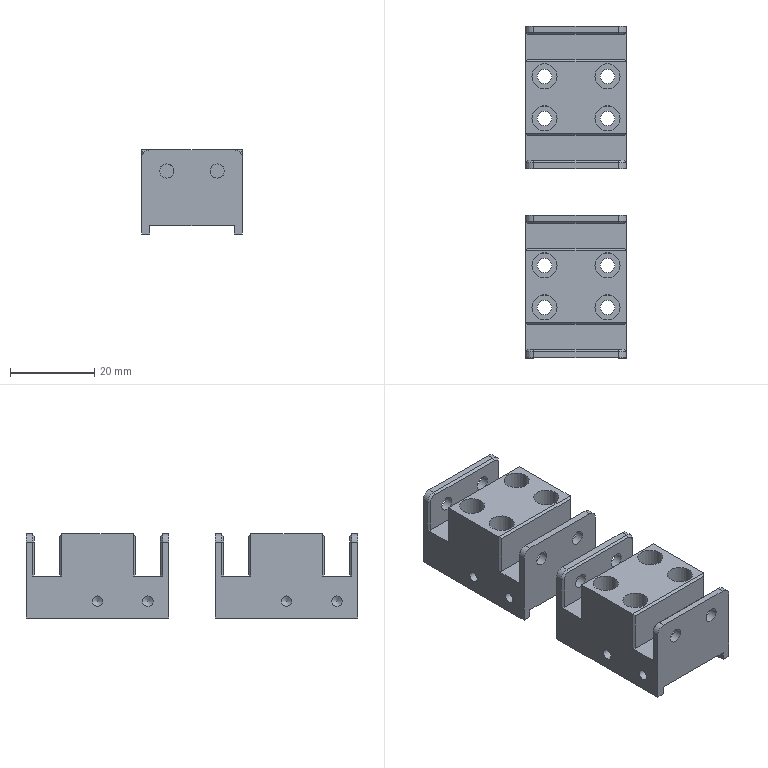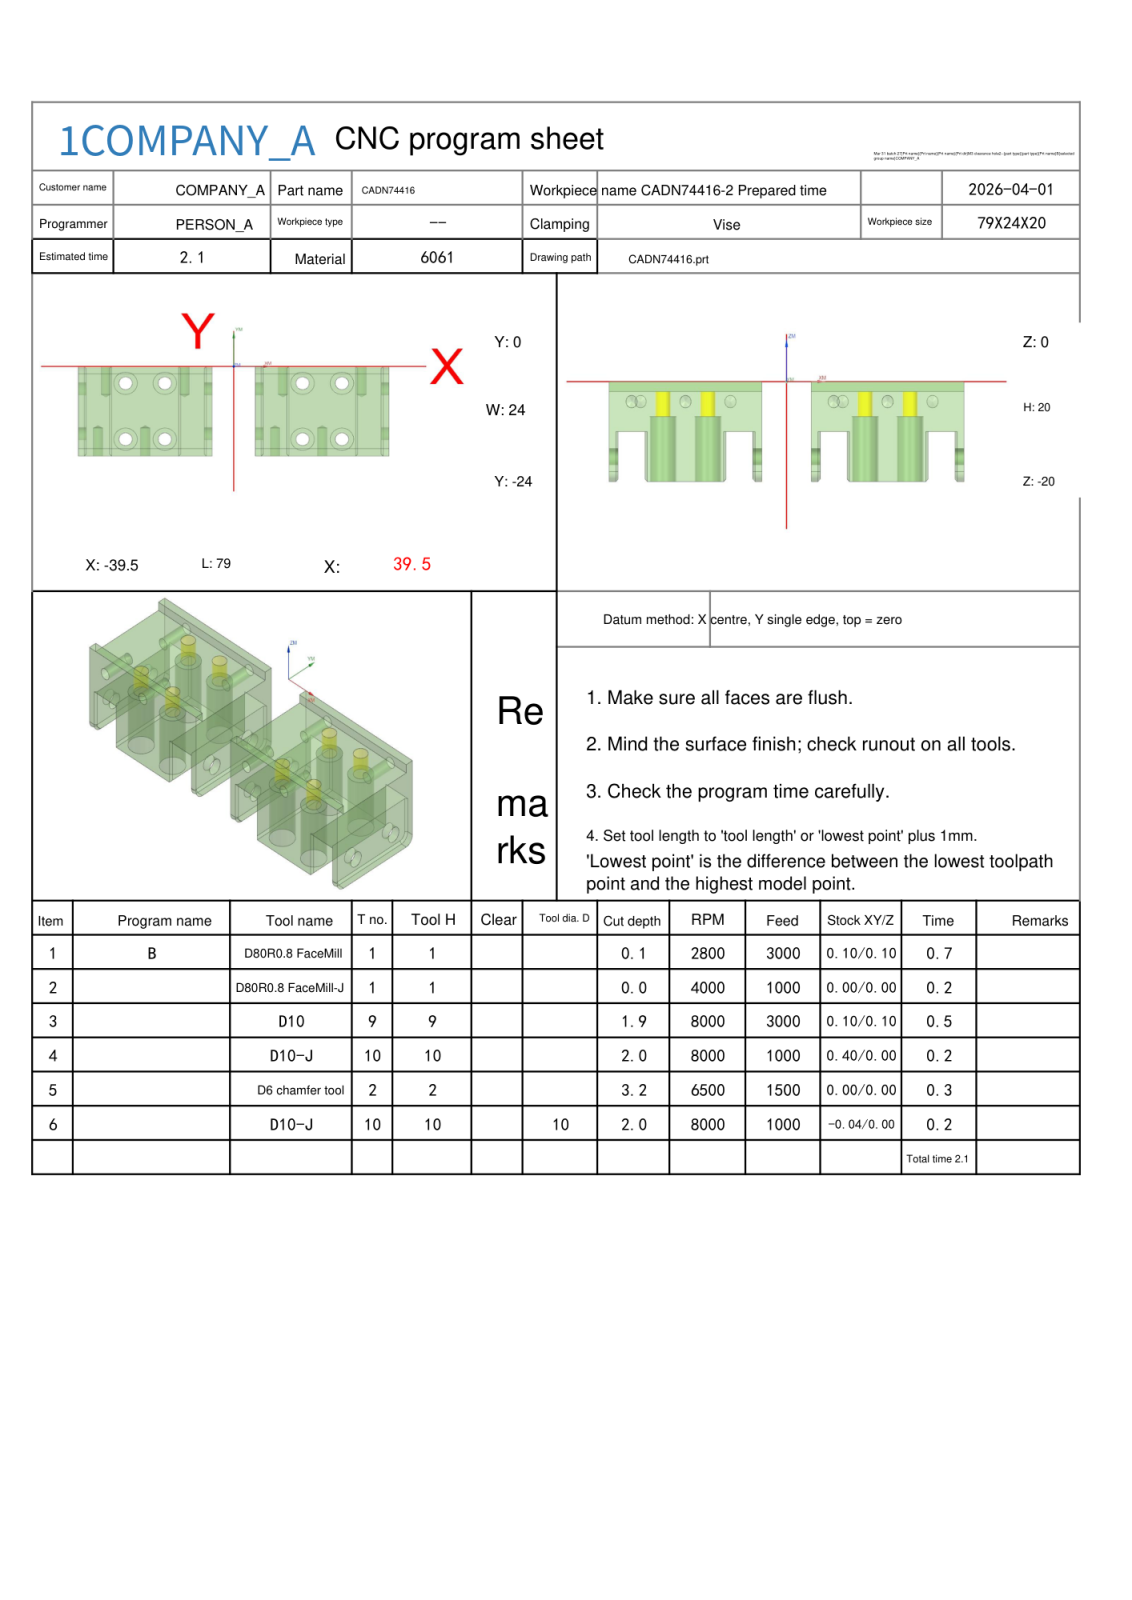NC program | NX | posted by the shop | part box 24 x 79 x 20 mm
Whole program:
%
O0001
(Machine time: 3.29 MIN)
(===Total Tool:4===)
(T1=D80R0.8 FaceMill D=80.  R=0.8  D-  H01 Z=0.    )
(T9=D10     D=10.  R=0.   D-  H09 Z=-1.9  )
(T10=D10-J  D=10.  R=0.   D-  H10 Z=-2.   )
(T2=D6 chamfer tool   D=6.   R=0.   D-  H02 Z=-3.2  )
G80 G90 G17 G49 G40
G91 G28 Z0
M01
N1 T01 M06
(D80R0.8 FaceMill  D=80. R=0.8 H=01 ce=0.10 di=0.10)
G00 G90 G54 X-91.597 Y-12. M03 S2800
G43 H01 Z20.
M08
Z6.011
G01 Z4.011 F3000.
X-79.597
X79.597
X91.597
Z6.011
G00 X-91.597
Z5.522
G01 Z3.522
X-79.597
X79.597
X91.597
Z5.522
G00 X-91.597
Z5.033
G01 Z3.033
X-79.597
X79.597
X91.597
Z5.033
G00 X-91.597
Z4.544
G01 Z2.544
X-79.597
X79.597
X91.597
Z4.544
G00 Z20.
X-91.597
Z4.056
G01 Z2.056
X-79.597
X79.597
X91.597
Z4.056
G00 Z20.
X-91.597
Z3.567
G01 Z1.567
X-79.597
X79.597
X91.597
Z3.567
G00 Z20.
X-91.597
Z3.078
G01 Z1.078
X-79.597
X79.597
X91.597
Z3.078
G00 Z20.
X-91.597
Z2.589
G01 Z.589
X-79.597
X79.597
X91.597
Z2.589
G00 Z20.
X-91.597
Z2.1
G01 Z.1
X-79.597
X79.597
X91.597
Z2.1
G00 Z20.
G91 G28 Z0.0
M05
M09
G91 G28 Z0.0
M01
N2 T01 M06
(D80R0.8 FaceMill-J  D=80. R=0.8 H=01 ce=0.00 di=0.00)
G00 G90 G54 X-91.499 Y-12. M03 S4000
G43 H01 Z20.
M08
Z2.
G01 Z0.0 F1000.
X-79.499
X79.499
X91.499
Z2.
G00 Z20.
G91 G28 Z0.0
M05
M09
G91 G28 Z0.0
M01
N3 T09 M06
(D10  D=10. R=0. H=09 ce=0.10 di=0.10)
G00 G90 G54 X47.5 Y-12. M03 S8000
G43 H09 Z14.5
M08
Z1.025
G01 Z-.475 F3000.
X44.4
Y-16.9
X-44.4
Y-7.1
X44.4
Y-9.132
G02 X43.848 Y-10.026 I-1. J0.0
G01 X40.253 Y-11.825
G03 X39.843 Y-12.205 I.448 J-.894
G02 X39.502 Y-12.4 I-.343 J.205
G01 X-39.502
G02 X-39.9 Y-12. I.002 J.4
X-39.502 Y-11.6 I.4 J0.0
G01 X39.502
G02 X39.9 Y-12. I-.002 J-.4
G01 Y-12.002
G02 X39.626 Y-12.38 I-.4 J.002
G01 X40.572 Y-15.227
X47.6
Z1.025
G00 X47.5 Y-12.
Z.55
G01 Z-.95
X44.4
Y-16.9
X-44.4
Y-7.1
X44.4
Y-9.132
G02 X43.848 Y-10.026 I-1. J0.0
G01 X40.253 Y-11.825
G03 X39.843 Y-12.205 I.448 J-.894
G02 X39.502 Y-12.4 I-.343 J.205
G01 X-39.502
G02 X-39.9 Y-12. I.002 J.4
X-39.502 Y-11.6 I.4 J0.0
G01 X39.502
G02 X39.9 Y-12. I-.002 J-.4
G01 Y-12.002
G02 X39.626 Y-12.38 I-.4 J.002
G01 X40.572 Y-15.227
X47.6
Z.55
G00 X47.5 Y-12.
Z.075
G01 Z-1.425
X44.4
Y-16.9
X-44.4
Y-7.1
X44.4
Y-9.132
G02 X43.848 Y-10.026 I-1. J0.0
G01 X40.253 Y-11.825
G03 X39.843 Y-12.205 I.448 J-.894
G02 X39.502 Y-12.4 I-.343 J.205
G01 X-39.502
G02 X-39.9 Y-12. I.002 J.4
X-39.502 Y-11.6 I.4 J0.0
G01 X39.502
G02 X39.9 Y-12. I-.002 J-.4
G01 Y-12.002
G02 X39.626 Y-12.38 I-.4 J.002
G01 X40.572 Y-15.227
X47.6
Z.075
G00 X47.5 Y-12.
Z-.4
G01 Z-1.9
X44.4
Y-16.9
X-44.4
Y-7.1
X44.4
Y-9.132
G02 X43.848 Y-10.026 I-1. J0.0
G01 X40.253 Y-11.825
G03 X39.843 Y-12.205 I.448 J-.894
G02 X39.502 Y-12.4 I-.343 J.205
G01 X-39.502
G02 X-39.9 Y-12. I.002 J.4
X-39.502 Y-11.6 I.4 J0.0
G01 X39.502
G02 X39.9 Y-12. I-.002 J-.4
G01 Y-12.002
G02 X39.626 Y-12.38 I-.4 J.002
G01 X40.572 Y-15.227
X47.6
Z-.4
G00 Z14.5
G91 G28 Z0.0
M05
M09
G91 G28 Z0.0
M01
N4 T10 M06
(D10-J  D=10. R=0. H=10 ce=0.40 di=0.00)
G00 G90 G54 X46.5 Y-10. M03 S8000
G43 H10 Z14.5
M08
Z-.5
G01 Z-2. F1000.
X42.5
G03 X40.5 Y-12. I0.0 J-2.
G01 Y-15.603
G02 X39.503 Y-16.6 I-1. J.003
G01 X-39.503
G02 X-40.5 Y-15.603 I.003 J1.
G01 Y-8.397
G02 X-39.503 Y-7.4 I1. J-.003
G01 X39.503
G02 X40.5 Y-8.397 I-.003 J-1.
G01 Y-12.
Y-13.
G03 X42.5 Y-15. I2. J0.0
G01 X46.9
Z-.5
G00 Z14.5
G91 G28 Z0.0
M05
M09
G91 G28 Z0.0
M01
N5 T02 M06
(D6 chamfer tool  D=6. R=0. H=02 ce=0.00 di=0.00)
G00 G90 G54 X22.114 Y1.227 M03 S6500
G43 H02 Z20.
M08
Z.172
G01 Z-1.2 F1500.
G03 X22.4 Y1.027 I1.286 J1.532
G01 X22.446 Y.997
X22.5 Y1.
X39.5
G02 X40.5 Y0.0 I0.0 J-1.
G01 Y-2.
G02 X39.5 Y-3. I-1. J0.0
G01 X5.5
G02 X4.5 Y-2. I0.0 J1.
G01 Y0.0
G02 X5.5 Y1. I1. J0.0
G01 X22.5
X22.554 Y.997
X22.6 Y1.027
G03 X22.886 Y1.227 I-1. J1.732
G01 Z.172
G00 Z10.
Y-25.227
Z.172
G01 Z-1.2
G03 X22.6 Y-25.027 I-1.286 J-1.532
G01 X22.554 Y-24.997
X22.5 Y-25.
X5.5
G02 X4.5 Y-24. I0.0 J1.
G01 Y-22.
G02 X5.5 Y-21. I1. J0.0
G01 X39.5
G02 X40.5 Y-22. I0.0 J-1.
G01 Y-24.
G02 X39.5 Y-25. I-1. J0.0
G01 X22.5
X22.446 Y-24.997
X22.4 Y-25.027
G03 X22.114 Y-25.227 I1. J-1.732
G01 Z.172
G00 Z10.
X-22.886 Y1.227
Z.172
G01 Z-1.2
G03 X-22.6 Y1.027 I1.286 J1.532
G01 X-22.554 Y.997
X-22.5 Y1.
X-5.5
G02 X-4.5 Y0.0 I0.0 J-1.
G01 Y-2.
G02 X-5.5 Y-3. I-1. J0.0
G01 X-39.5
G02 X-40.5 Y-2. I0.0 J1.
G01 Y0.0
G02 X-39.5 Y1. I1. J0.0
G01 X-22.5
X-22.446 Y.997
X-22.4 Y1.027
G03 X-22.114 Y1.227 I-1. J1.732
G01 Z.172
G00 Z10.
Y-25.227
Z.172
G01 Z-1.2
G03 X-22.4 Y-25.027 I-1.286 J-1.532
G01 X-22.446 Y-24.997
X-22.5 Y-25.
X-39.5
G02 X-40.5 Y-24. I0.0 J1.
G01 Y-22.
G02 X-39.5 Y-21. I1. J0.0
G01 X-5.5
G02 X-4.5 Y-22. I0.0 J-1.
G01 Y-24.
G02 X-5.5 Y-25. I-1. J0.0
G01 X-22.5
X-22.554 Y-24.997
X-22.6 Y-25.027
G03 X-22.886 Y-25.227 I1. J-1.732
G01 Z.172
G00 Z10.
X-40.568 Y-19.03
Z-1.669
G01 Z-3.2
X-40.508 Y-18.944
X-40.5 Y-18.914
Y-5.086
X-40.508 Y-5.056
X-40.568 Y-4.97
Z-1.669
G00 Z10.
X-4.432
Z-1.669
G01 Z-3.2
X-4.492 Y-5.056
X-4.5 Y-5.086
Y-18.914
X-4.492 Y-18.944
X-4.432 Y-19.03
Z-1.669
G00 Z10.
X40.568 Y-4.97
Z-1.669
G01 Z-3.2
X40.508 Y-5.056
X40.5 Y-5.086
Y-18.914
X40.508 Y-18.944
X40.568 Y-19.03
Z-1.669
G00 Z10.
X4.432
Z-1.669
G01 Z-3.2
X4.492 Y-18.944
X4.5 Y-18.914
Y-5.086
X4.492 Y-5.056
X4.432 Y-4.97
Z-1.669
G00 Z20.
G91 G28 Z0.0
M05
M09
G91 G28 Z0.0
M01
N6 T10 M06
(D10-J  D=10. R=0. H=10 ce=-0.04 di=0.00)
G00 G90 G54 X46.502 Y-8.789 M03 S8000
G43 H10 Z14.5
M08
Z-1.
G01 Z-2. F1000.
G41 D10
X46.465 Y-8.592
G03 X44.5 Y-6.965 I-1.965 J-.373
G01 X-44.5
G03 X-46.465 Y-8.592 I0.0 J-2.
G01 G40 X-46.502 Y-8.789
Y-15.211
G41 D10
X-46.465 Y-15.408
G03 X-44.5 Y-17.035 I1.965 J.373
G01 X44.5
G03 X46.465 Y-15.408 I0.0 J2.
G01 G40 X46.502 Y-15.211
Z-1.
G00 Z14.5
M05
M09
G91 G28 Z0.0
G91 G28 Y0.0
M30
%